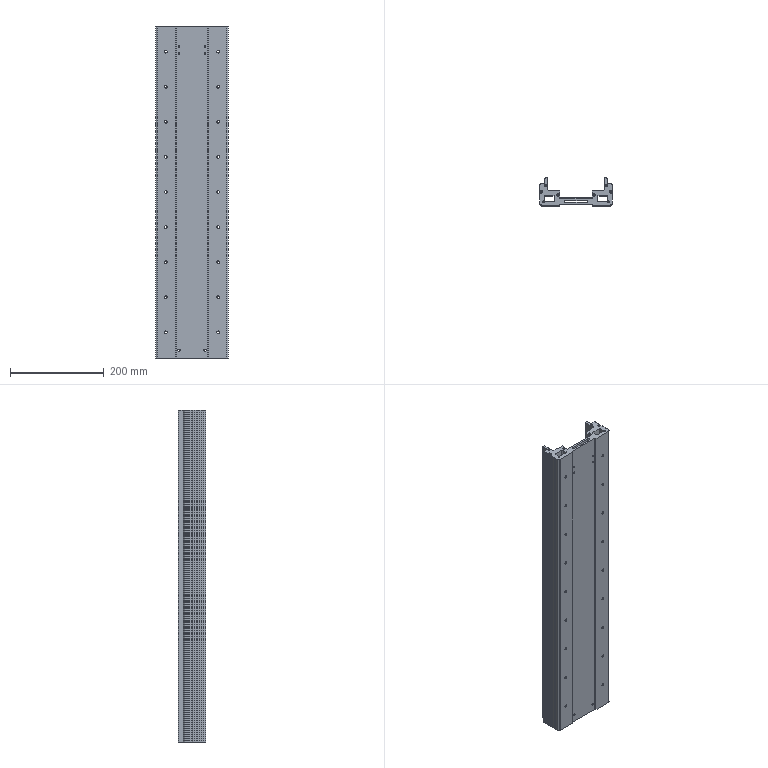Part | STEP file | 1 solid | 290 faces | box 155 x 59.25 x 710 mm | volume 2291681 mm3 | plane 154 | cylinder 113 | cone 23 | commonest cylinder face diameters 3.3 x27 5.5 x18 9 x18 2 x12 0.5 x8 4 x8